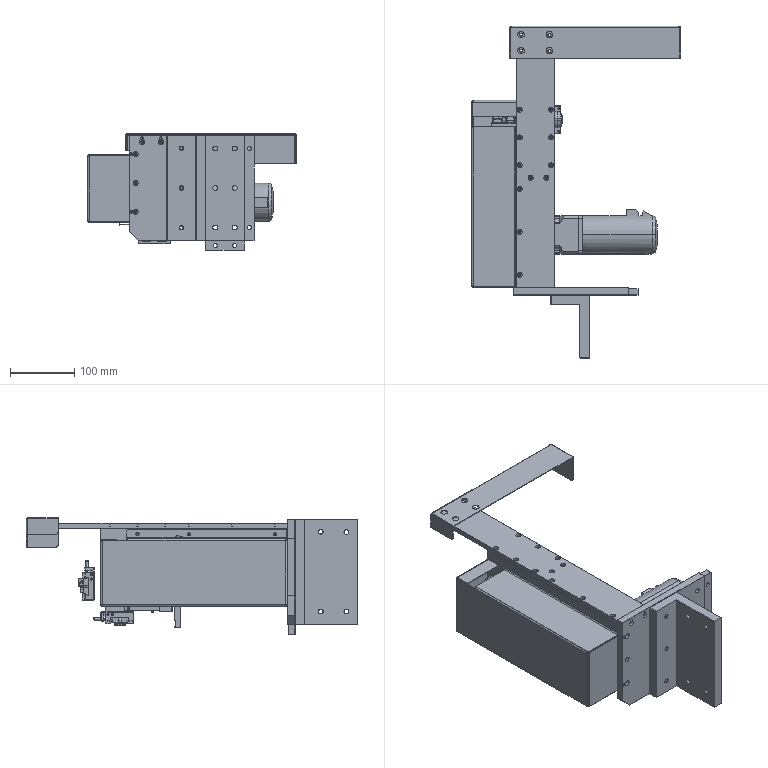Part | NX | 79 solids | 4547 faces | volume 2410078 mm3 | plane 1995 | cylinder 1705 | cone 634 | torus 126 | sphere 60 | spline 27 | commonest cylinder face diameters 2.5 x250 3.3 x163 0.5 x97 6.55 x97 1.1 x93 4.5 x86